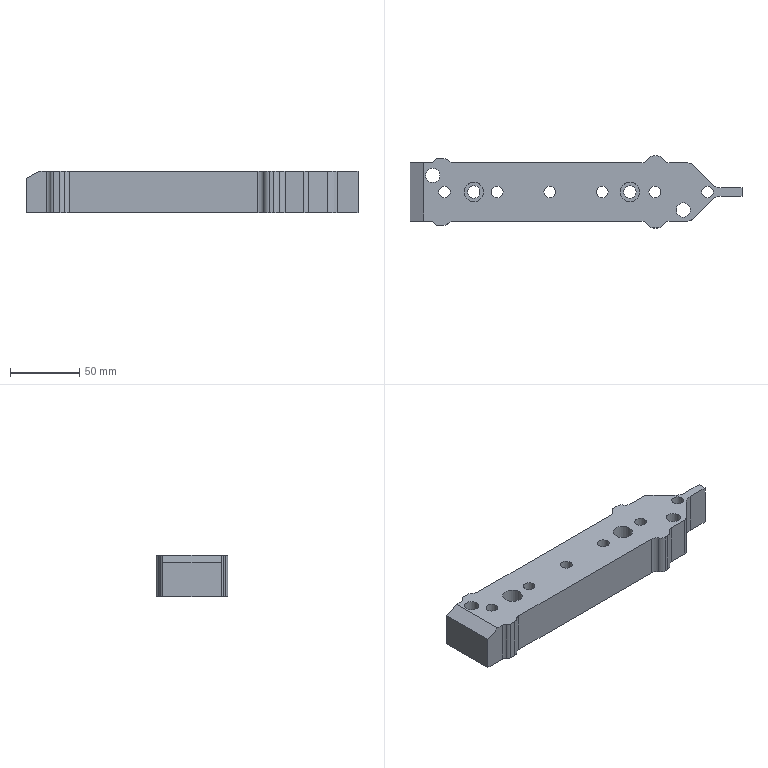Part | STEP file | 1 solid | 57 faces | box 240 x 52 x 30 mm | volume 250447 mm3 | cylinder 34 | plane 23 | commonest cylinder face diameters 10 x12 8.5 x6 6 x4 9 x4 20 x4 10.306 x2